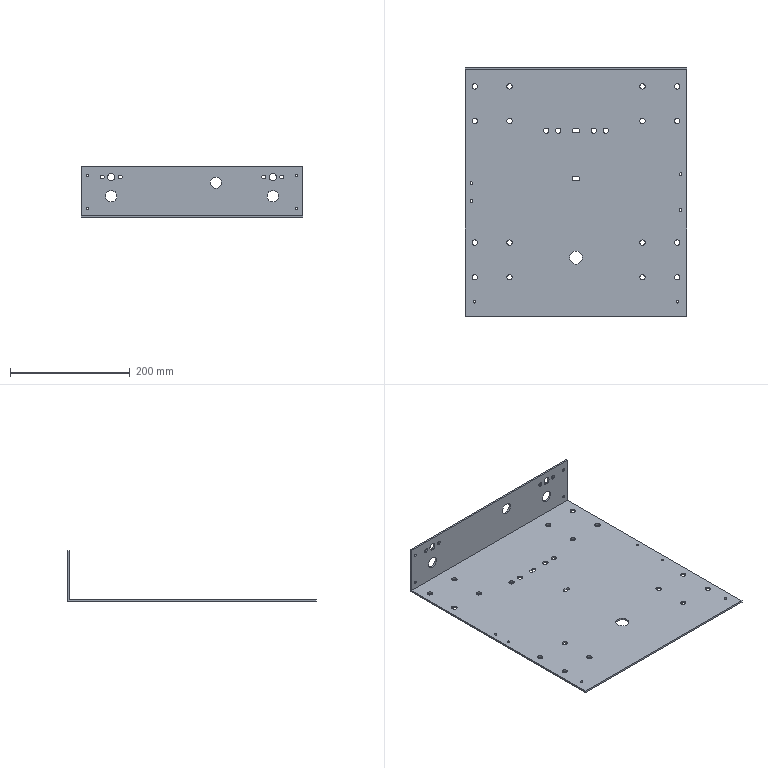Part | STEP file | 601-01-0067 | 1 solid | 98 faces | box 370 x 415 x 85 mm | volume 542185 mm3 | cylinder 86 | plane 12 | commonest cylinder face diameters 9 x40 4.2 x20 6.5 x8 7 x6 19 x6 12 x4